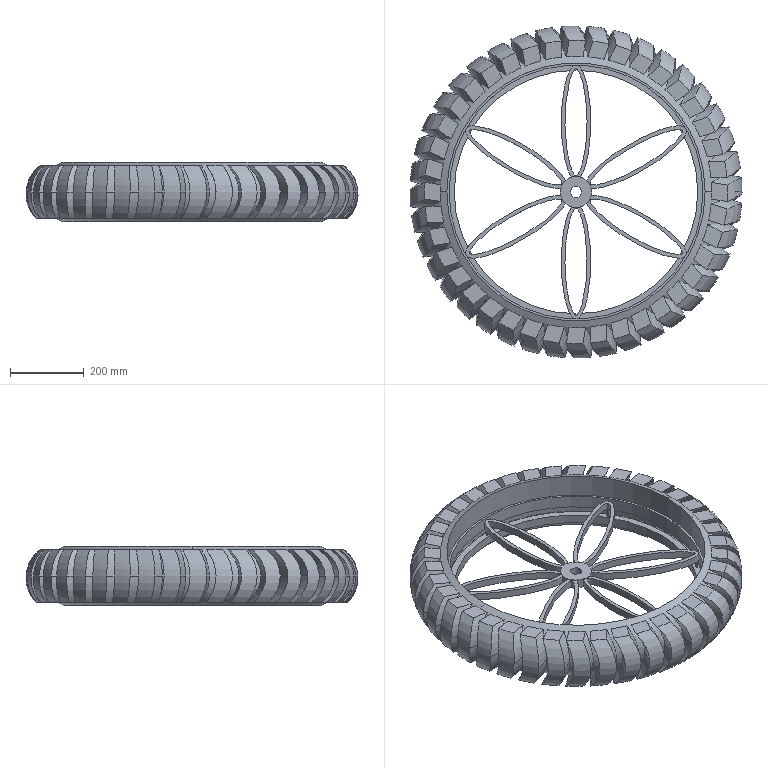Part | SolidWorks | features ICE 5, CirPattern 4, BossThin 1, ExtruThin 1, Fillet 1, RefAxis 1, RevCut 1, Revolution 1 | 2 solids | 443 faces | box 900 x 900 x 159.998 mm | volume 29745810 mm3 | cylinder 266 | plane 110 | torus 49 | spline 18 | commonest cylinder face diameters 219.086 x156 64.33 x40 710 x40 5 x18 700 x4 30 x2